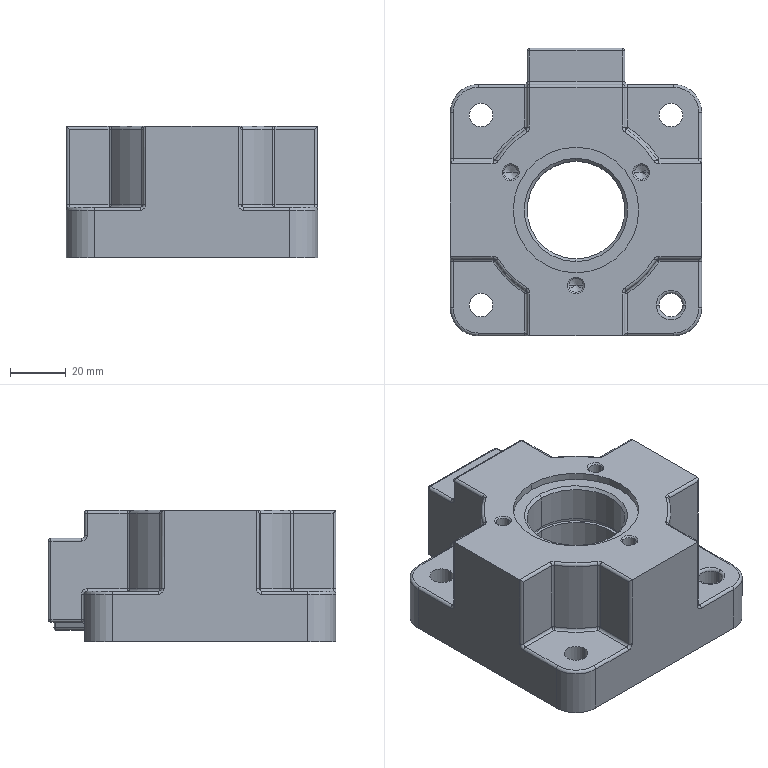Part | SolidWorks | features 3DProfileFeature 3, Fillet 3, HoleWzd 3, ICE 3, Chamfer 1, Extrusion 1, RevCut 1 | 1 solid | 210 faces | box 90 x 103 x 47 mm | volume 196291 mm3 | cylinder 98 | torus 34 | plane 33 | cone 30 | sphere 15 | commonest cylinder face diameters 2 x57 8.5 x8 5 x6 20 x4 35 x4 68 x4